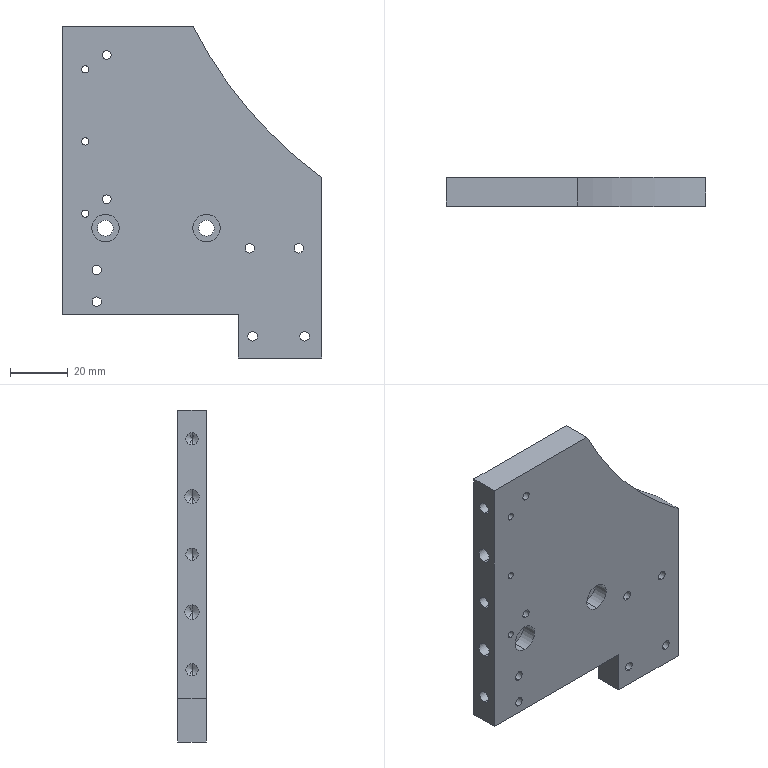Part | STEP file | PN_0003 | 1 solid | 61 faces | box 90 x 10 x 115 mm | volume 78081 mm3 | cylinder 41 | cone 10 | plane 10 | commonest cylinder face diameters 3.3 x12 2.5 x6 4.2 x6 3 x4 5 x4 5.5 x4